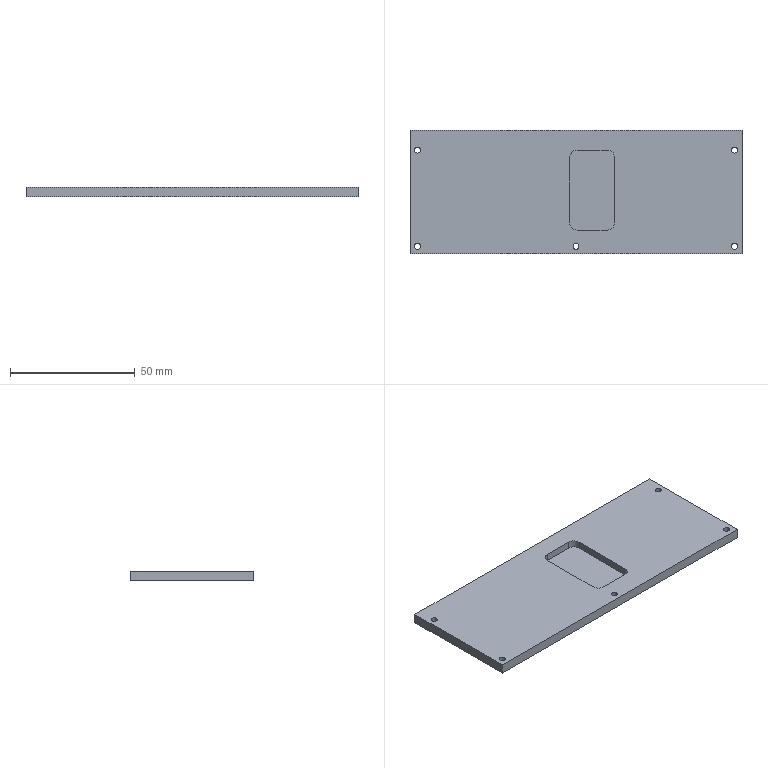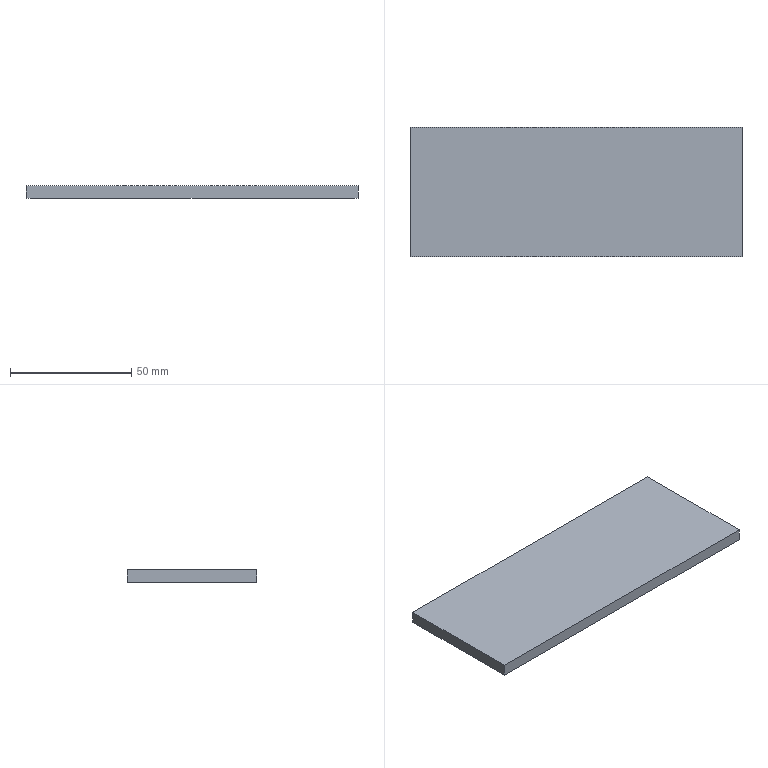CAM job | NX | 3-axis milling, drilling | part box 133 x 49.5 x 4 mm | stock box 137 x 53.5 x 5 mm
Tools:
number,name,description,diameter,corner_radius,flute_length,length,flutes
9,D10JING,Milling Tool-5 Parameters,10.0,0.0,50.0,75.0,2
7,D6A45,Milling Tool-5 Parameters,6.0,0.0,50.0,75.0,2
6,D6,Milling Tool-5 Parameters,6.0,0.0,50.0,75.0,2
14,2.4ZT,Drilling Tool,2.4,0.0,35.0,50.0,2
3,D3,Milling Tool-5 Parameters,3.0,0.0,50.0,75.0,2
Operations:
program,operation,operation_type,tool,method,geometry_group,spindle_rpm,surface_speed,feed_per_tooth,feed_cut,feed_plunge,cut_length_mm,path_length_mm,cut_time_min,machine_time_min
1,FLOOR_WALL,VolumeBased25DMillingOperation,D10JING,METHOD,A,9500.0,298.0,0.0658,1250.0,100.0,1678.497,1732.497,1.343,1.348
1,DRILLING,Operation,D6A45,METHOD,A,5000.0,94.0,0.025,250.0,0.0,21.5,319.375,0.086,0.1158
1,DRILLING_COPY,Operation,2.4ZT,METHOD,A,2000.0,15.0,0.0375,150.0,0.0,41.105,358.585,0.274,0.3058
1,ZLEVEL_PROFILE,ZLevelMilling,D6,METHOD,A,9500.0,298.0,0.1316,2500.0,1000.0,5051.03,5111.88,2.041,2.047
1,FLOOR_WALL_1,VolumeBased25DMillingOperation,D6,METHOD,A,9500.0,298.0,0.1316,2500.0,1000.0,1873.485,2002.537,0.8973,0.9102
1,FLOOR_WALL_1_COPY,VolumeBased25DMillingOperation,D6,METHOD,A,9500.0,298.0,0.0632,1200.0,1000.0,244.472,308.472,0.2041,0.2105
1,ZLEVEL_PROFILE_1_COPY,ZLevelMilling,D6A45,METHOD,A,9500.0,179.0,0.0658,1250.0,100.0,507.518,1436.982,0.406,0.499
1,刀补,ZLevelMilling,D6,METHOD,A,9500.0,89.0,0.0632,1200.0,1000.0,390.253,454.953,0.3257,0.3322
2,HOLE_MILLING,CylinderMilling,D3,METHOD,B,9500.0,89.0,0.0658,1250.0,100.0,317.111,840.871,0.2537,0.3061
2,ZLEVEL_PROFILE_1_COPY_COPY,ZLevelMilling,D6A45,METHOD,B,9500.0,179.0,0.0658,1250.0,100.0,439.083,1312.287,0.3513,0.4386